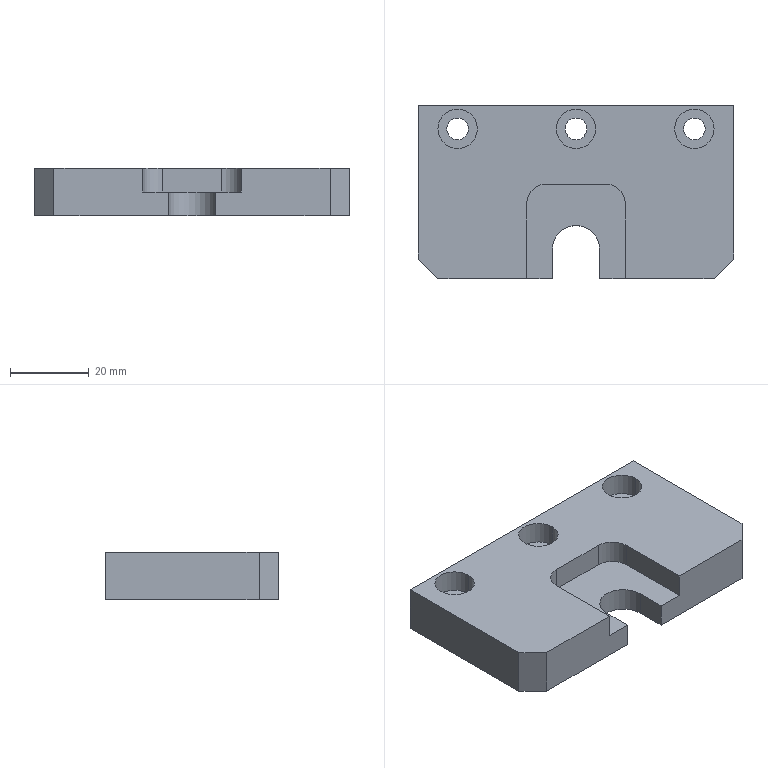Part | STEP file | PN_0087 transport cylinder connecting plate | 1 solid | 33 faces | box 80 x 44 x 12 mm | volume 35733 mm3 | plane 18 | cylinder 15 | commonest cylinder face diameters 10 x8 5.5 x6 12 x1